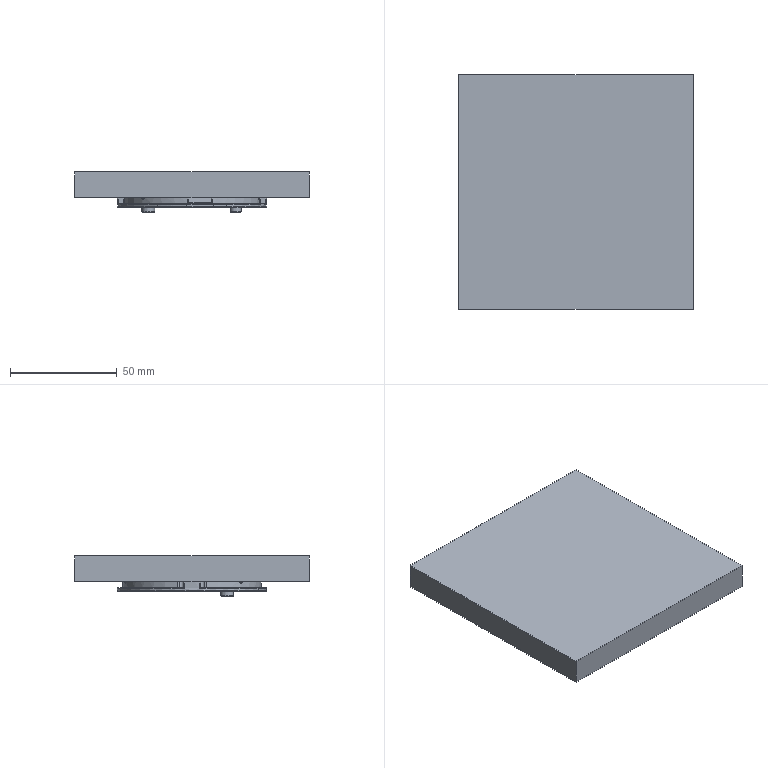NC program | NX | posted with a generic post | part box 110 x 110 x 18.8 mm
Lines 1 to 1072 of 3099:
N10 G17 G21 G94 G90
(FLOOR_WALL_COPY_1 , TOOL : D10)
N12 T04 M6
N14 G54
N16 G17 G0 G90 X-63. Y54.997 S6500 M3
N18 G43 Z30. H4
N20 Z3.
N22 G94 G1 Z0. F1250.
N24 X-60.
N26 X60.
N28 Y47.426
N30 X-60.
N32 Y39.855
N34 X60.
N36 Y32.283
N38 X-60.
N40 Y24.712
N42 X60.
N44 Y17.141
N46 X-60.
N48 Y9.57
N50 X60.
N52 Y1.999
N54 X-60.
N56 Y-5.573
N58 X60.
N60 Y-13.144
N62 X-60.
N64 Y-20.715
N66 X60.
N68 Y-28.286
N70 X-60.
N72 Y-35.858
N74 X60.
N76 Y-43.429
N78 X-60.
N80 Y-51.
N82 X60.
N84 X63.
N86 Z3.
N88 G0 Z30.
(FLOOR_WALL_COPY_1_COPY , TOOL : D10)
N90 X-20.7 Y1.195 S9500
N92 Z2.5
N94 G1 Y22.11 Z1.404 F1000.
N96 X-20.385 Y23.534 Z1.327
N98 X-19.742 Y24.842 Z1.251
N100 X-18.809 Y25.962 Z1.174
N102 X-18.329 Y26.332 Z1.143
N104 X-18.112 Y26.5 Z1.128
N106 X-26.5 Z0.689
N108 Y0. Z-0.7
N110 Y-26.5 F2500.
N112 X-19.233
N114 G2 X-20.7 Y-22.532 R6.1
N116 G1 Y21.505
N118 G2 X-18.329 Y26.332 R6.1
N120 G1 X-18.112 Y26.5
N122 X-26.5
N124 Y0.
N126 X-31.
N128 Y-31.
N130 X3.393
N132 X9.837 Y-33.606
N134 X3.393 Y-31.
N136 X-15.163 Y-24.03
N138 G2 X-16.2 Y-22.532 R1.6
N140 G1 Y21.505
N142 G2 X-15.578 Y22.771 R1.6
N144 G1 X-4.926 Y31.
N146 X-3.948 Y29.734
N148 X1.111 Y33.642
N150 X3.111 Y33.456
N152 G2 X12.353 Y-31.247 R33.6
N154 G1 X10.525 Y-31.97
N156 X-14.6 Y-22.532
N158 Y21.505
N160 X-3.948 Y29.734
N162 X-4.926 Y31.
N164 X-31.
N166 Y0.
N168 X-39.
N170 Y-39.
N172 X16.675
N174 Y-31.
N176 X31.
N178 Y-16.675
N180 X33.692 Y-11.317
N182 X31. Y-16.675
N184 G2 X16.675 Y-31. R35.2
N186 G1 Y-39.
N188 X39.
N190 Y16.675
N192 X31.
N194 Y31.
N196 X16.675
N198 X11.317 Y33.692
N200 X16.675 Y31.
N202 G2 X31. Y16.675 R35.2
N204 G1 X33.692 Y11.317
N206 X31. Y16.675
N208 X39.
N210 Y39.
N212 X-39.
N214 Y0.
N216 X-47.
N218 Y-47.
N220 X47.
N222 Y47.
N224 X-47.
N226 Y0.
N228 X-55.
N230 Y-47.988
N232 Y-55.
N234 X55.
N236 Y55.
N238 X-55.
N240 Y0.
N242 Z0.8
N244 G0 X-20.7 Y1.199
N246 G1 Y21.505 Z-0.264 F1000.
N248 Y22.11 Z-0.296
N250 X-20.389 Y23.521 Z-0.372
N252 X-19.879 Y24.62 Z-0.435
N254 X-19.391 Y25.329 Z-0.48
N256 X-18.809 Y25.962 Z-0.525
N258 X-18.112 Y26.5 Z-0.572
N260 X-26.5 Z-1.011
N262 Y0. Z-2.4
N264 Y-26.5 F2500.
N266 X-19.233
N268 G2 X-20.7 Y-22.532 R6.1
N270 G1 Y21.505
N272 G2 X-18.329 Y26.332 R6.1
N274 G1 X-18.112 Y26.5
N276 X-26.5
N278 Y0.
N280 X-31.
N282 Y-31.
N284 X3.393
N286 X9.837 Y-33.606
N288 X3.393 Y-31.
N290 X-15.163 Y-24.03
N292 G2 X-16.2 Y-22.532 R1.6
N294 G1 Y21.505
N296 G2 X-15.578 Y22.771 R1.6
N298 G1 X-4.926 Y31.
N300 X-3.948 Y29.734
N302 X1.111 Y33.642
N304 X3.111 Y33.456
N306 G2 X12.353 Y-31.247 R33.6
N308 G1 X10.525 Y-31.97
N310 X-14.6 Y-22.532
N312 Y21.505
N314 X-3.948 Y29.734
N316 X-4.926 Y31.
N318 X-31.
N320 Y0.
N322 X-39.
N324 Y-39.
N326 X16.675
N328 Y-31.
N330 X31.
N332 Y-16.675
N334 X33.692 Y-11.317
N336 X31. Y-16.675
N338 G2 X16.675 Y-31. R35.2
N340 G1 Y-39.
N342 X39.
N344 Y16.675
N346 X31.
N348 Y31.
N350 X16.675
N352 X11.317 Y33.692
N354 X16.675 Y31.
N356 G2 X31. Y16.675 R35.2
N358 G1 X33.692 Y11.317
N360 X31. Y16.675
N362 X39.
N364 Y39.
N366 X-39.
N368 Y0.
N370 X-47.
N372 Y-47.
N374 X47.
N376 Y47.
N378 X-47.
N380 Y0.
N382 X-55.
N384 Y-55.
N386 X55.
N388 Y55.
N390 X-55.
N392 Y0.
N394 Z-0.9
N396 G0 Z30.
(CAVITY_MILL_COPY , TOOL : D10)
N398 X-20.6 Y-3.644
N400 Z-1.
N402 G1 Y5.416 Z-1.475 F1000.
N404 X-20.888 Y4.322 Z-1.534
N406 X-21.281 Y1.45 Z-1.686
N408 Y-1.45 Z-1.838
N410 X-20.888 Y-4.322 Z-1.99
N412 X-20.6 Y-5.416 Z-2.049
N414 Y5.416 Z-2.617
N416 X-20.888 Y4.322 Z-2.676
N418 X-21.281 Y1.45 Z-2.828
N420 Y-1.45 Z-2.98
N422 X-20.888 Y-4.322 Z-3.132
N424 X-20.6 Y-5.416 Z-3.191
N426 Y0. Z-3.475
N428 Y5.416 F3000.
N430 X-19.652 Y10.432
N432 X-20.6 Y5.416
N434 G3 X-20.6 Y-5.416 R21.3
N436 G1 X-19.652 Y-10.432
N438 X-20.6 Y-5.416
N440 Y0.
N442 X-14.6
N444 Y19.
N446 G2 X-12.618 Y23.036 R5.1
N448 G1 X-9.136 Y25.726
N450 G3 X-2.128 Y-27.217 R27.3
N452 G1 X-11.293 Y-23.774
N454 G2 X-14.6 Y-19. R5.1
N456 G1 Y0.
N458 G3 X-15.1 Y0.866 R1.
N460 G1 Z-1.975
N462 G0 Z30.
N464 X-20.6 Y-3.644
N466 Z-1.975
N468 G1 Y5.416 Z-2.45 F1000.
N470 X-20.888 Y4.322 Z-2.509
N472 X-21.281 Y1.45 Z-2.661
N474 Y-1.45 Z-2.813
N476 X-20.888 Y-4.322 Z-2.965
N478 X-20.6 Y-5.416 Z-3.024
N480 Y5.416 Z-3.592
N482 X-20.888 Y4.322 Z-3.651
N484 X-21.281 Y1.45 Z-3.803
N486 Y-1.45 Z-3.955
N488 X-20.888 Y-4.322 Z-4.107
N490 X-20.6 Y-5.416 Z-4.166
N492 Y0. Z-4.45
N494 Y5.416 F3000.
N496 X-19.652 Y10.432
N498 X-20.6 Y5.416
N500 G3 X-20.6 Y-5.416 R21.3
N502 G1 X-19.652 Y-10.432
N504 X-20.6 Y-5.416
N506 Y0.
N508 X-14.6
N510 Y19.
N512 G2 X-12.618 Y23.036 R5.1
N514 G1 X-9.136 Y25.726
N516 G3 X-2.128 Y-27.217 R27.3
N518 G1 X-11.293 Y-23.774
N520 G2 X-14.6 Y-19. R5.1
N522 G1 Y0.
N524 G3 X-15.1 Y0.866 R1.
N526 G1 Z-2.95
N528 G0 X-20.6 Y-3.644
N530 G1 Y5.416 Z-3.425 F1000.
N532 X-20.888 Y4.322 Z-3.484
N534 X-21.281 Y1.45 Z-3.636
N536 Y-1.45 Z-3.788
N538 X-20.888 Y-4.322 Z-3.94
N540 X-20.6 Y-5.416 Z-3.999
N542 Y5.416 Z-4.567
N544 X-20.888 Y4.322 Z-4.626
N546 X-21.281 Y1.45 Z-4.778
N548 Y-1.45 Z-4.93
N550 X-20.888 Y-4.322 Z-5.082
N552 X-20.6 Y-5.416 Z-5.141
N554 Y0. Z-5.425
N556 Y5.416 F3000.
N558 X-19.652 Y10.432
N560 X-20.6 Y5.416
N562 G3 X-20.6 Y-5.416 R21.3
N564 G1 X-19.652 Y-10.432
N566 X-20.6 Y-5.416
N568 Y0.
N570 X-14.6
N572 Y19.
N574 G2 X-12.618 Y23.036 R5.1
N576 G1 X-9.136 Y25.726
N578 G3 X-2.128 Y-27.217 R27.3
N580 G1 X-11.293 Y-23.774
N582 G2 X-14.6 Y-19. R5.1
N584 G1 Y0.
N586 G3 X-15.1 Y0.866 R1.
N588 G1 Z-3.925
N590 G0 X-20.6 Y-3.644
N592 G1 Y5.416 Z-4.4 F1000.
N594 X-20.888 Y4.322 Z-4.459
N596 X-21.281 Y1.45 Z-4.611
N598 Y-1.45 Z-4.763
N600 X-20.888 Y-4.322 Z-4.915
N602 X-20.6 Y-5.416 Z-4.974
N604 Y5.416 Z-5.542
N606 X-20.888 Y4.322 Z-5.601
N608 X-21.281 Y1.45 Z-5.753
N610 Y-1.45 Z-5.905
N612 X-20.888 Y-4.322 Z-6.057
N614 X-20.6 Y-5.416 Z-6.116
N616 Y0. Z-6.4
N618 Y5.416 F3000.
N620 X-19.652 Y10.432
N622 X-20.6 Y5.416
N624 G3 X-20.6 Y-5.416 R21.3
N626 G1 X-19.652 Y-10.432
N628 X-20.6 Y-5.416
N630 Y0.
N632 X-14.6
N634 Y19.
N636 G2 X-12.618 Y23.036 R5.1
N638 G1 X-9.136 Y25.726
N640 G3 X-2.128 Y-27.217 R27.3
N642 G1 X-11.293 Y-23.774
N644 G2 X-14.6 Y-19. R5.1
N646 G1 Y0.
N648 G3 X-15.1 Y0.866 R1.
N650 G1 Z-4.9
N652 G0 X-16.803 Y-13.9
N654 G1 X-14.6 Z-5.015 F1000.
N656 Y13.9 Z-6.472
N658 X-18.4 Z-6.672
N660 Y0. Z-7.4
N662 Y-13.9 F3000.
N664 X-14.6
N666 Y13.9
N668 X-18.4
N670 Y0.
N672 G3 X-17.9 Y-0.866 R1.
N674 G1 Z-5.9
N676 G0 X-16.803 Y-13.9
N678 G1 X-14.6 Z-6.015 F1000.
N680 Y13.9 Z-7.472
N682 X-18.4 Z-7.672
N684 Y0. Z-8.4
N686 Y-13.9 F3000.
N688 X-14.6
N690 Y13.9
N692 X-18.4
N694 Y0.
N696 G3 X-17.9 Y-0.866 R1.
N698 G1 Z-6.9
N700 G0 X-16.803 Y-13.9
N702 G1 X-14.6 Z-7.015 F1000.
N704 Y13.9 Z-8.472
N706 X-18.4 Z-8.672
N708 Y0. Z-9.4
N710 Y-13.9 F3000.
N712 X-14.6
N714 Y13.9
N716 X-18.4
N718 Y0.
N720 G3 X-17.9 Y-0.866 R1.
N722 G1 Z-7.9
N724 G0 X-16.803 Y-13.9
N726 G1 X-14.6 Z-8.015 F1000.
N728 Y13.9 Z-9.472
N730 X-18.4 Z-9.672
N732 Y0. Z-10.4
N734 Y-13.9 F3000.
N736 X-14.6
N738 Y13.9
N740 X-18.4
N742 Y0.
N744 G3 X-17.9 Y-0.866 R1.
N746 G1 Z-8.9
N748 G0 X-16.803 Y-13.9
N750 G1 X-14.6 Z-9.015 F1000.
N752 Y13.9 Z-10.472
N754 X-18.4 Z-10.672
N756 Y0. Z-11.4
N758 Y-13.9 F3000.
N760 X-14.6
N762 Y13.9
N764 X-18.4
N766 Y0.
N768 G3 X-17.9 Y-0.866 R1.
N770 G1 Z-9.9
N772 G0 Z30.
N774 M5
(CAVITY_MILL_COPY_1_COPY_1 , TOOL : D6)
N776 T16 M6
N778 G54
N780 G17 G0 G90 X-2.983 Y-28.042 S9500 M3
N782 G43 Z30. H16
N784 Z-2.
N786 G94 G1 Z-3. F1000.
N788 X-2.607 Y-28.795
N790 G3 X-1.773 Y-29.347 R1.
N792 X7.243 Y-28.494 R29.4 F1600.
N794 G1 X-0.959 Y-25.413
N796 G3 X-1.946 Y-25.576 R1.
N798 G1 X-2.57 Y-26.089
N800 Z-2.
N802 G0 Z30.
N804 X-2.983 Y-28.042
N806 Z-2.5
N808 G1 Z-3.5 F1000.
N810 X-2.607 Y-28.795
N812 G3 X-1.773 Y-29.347 R1.
N814 X7.243 Y-28.494 R29.4 F1600.
N816 G1 X-0.959 Y-25.413
N818 G3 X-1.946 Y-25.576 R1.
N820 G1 X-2.57 Y-26.089
N822 Z-2.5
N824 G0 X-2.983 Y-28.042 Z-3.
N826 G1 Z-4. F1000.
N828 X-2.607 Y-28.795
N830 G3 X-1.773 Y-29.347 R1.
N832 X7.243 Y-28.494 R29.4 F1600.
N834 G1 X-0.959 Y-25.413
N836 G3 X-1.946 Y-25.576 R1.
N838 G1 X-2.57 Y-26.089
N840 Z-3.
N842 G0 X-2.983 Y-28.042 Z-3.5
N844 G1 Z-4.5 F1000.
N846 X-2.607 Y-28.795
N848 G3 X-1.773 Y-29.347 R1.
N850 X7.243 Y-28.494 R29.4 F1600.
N852 G1 X-0.959 Y-25.413
N854 G3 X-1.946 Y-25.576 R1.
N856 G1 X-2.57 Y-26.089
N858 Z-3.5
N860 G0 X-2.983 Y-28.042 Z-4.
N862 G1 Z-5. F1000.
N864 X-2.607 Y-28.795
N866 G3 X-1.773 Y-29.347 R1.
N868 X7.243 Y-28.494 R29.4 F1600.
N870 G1 X-0.959 Y-25.413
N872 G3 X-1.946 Y-25.576 R1.
N874 G1 X-2.57 Y-26.089
N876 Z-4.
N878 G0 X-2.983 Y-28.042 Z-4.5
N880 G1 Z-5.5 F1000.
N882 X-2.607 Y-28.795
N884 G3 X-1.773 Y-29.347 R1.
N886 X7.243 Y-28.494 R29.4 F1600.
N888 G1 X-0.959 Y-25.413
N890 G3 X-1.946 Y-25.576 R1.
N892 G1 X-2.57 Y-26.089
N894 Z-4.5
N896 G0 X-2.983 Y-28.042 Z-5.
N898 G1 Z-6. F1000.
N900 X-2.607 Y-28.795
N902 G3 X-1.773 Y-29.347 R1.
N904 X7.243 Y-28.494 R29.4 F1600.
N906 G1 X-0.959 Y-25.413
N908 G3 X-1.946 Y-25.576 R1.
N910 G1 X-2.57 Y-26.089
N912 Z-5.
N914 G0 X-2.983 Y-28.042 Z-5.5
N916 G1 Z-6.5 F1000.
N918 X-2.607 Y-28.795
N920 G3 X-1.773 Y-29.347 R1.
N922 X7.243 Y-28.494 R29.4 F1600.
N924 G1 X-0.959 Y-25.413
N926 G3 X-1.946 Y-25.576 R1.
N928 G1 X-2.57 Y-26.089
N930 Z-5.5
N932 G0 Z30.
N934 X-15.987 Y-14.8
N936 Z-6.
N938 G1 Z-7. F1000.
N940 X-15.582 Y-15.5
N942 G3 X-14.716 Y-16. R1.
N944 G1 X-12.5 F1600.
N946 Y-13.784
N948 G3 X-13. Y-12.918 R1.
N950 G1 X-13.7 Y-12.513
N952 Z-6.
N954 G0 X-15.987 Y-14.8 Z-6.5
N956 G1 Z-7.5 F1000.
N958 X-15.582 Y-15.5
N960 G3 X-14.716 Y-16. R1.
N962 G1 X-12.5 F1600.
N964 Y-13.784
N966 G3 X-13. Y-12.918 R1.
N968 G1 X-13.7 Y-12.513
N970 Z-6.5
N972 G0 X-15.987 Y-14.8 Z-7.
N974 G1 Z-8. F1000.
N976 X-15.582 Y-15.5
N978 G3 X-14.716 Y-16. R1.
N980 G1 X-12.5 F1600.
N982 Y-13.784
N984 G3 X-13. Y-12.918 R1.
N986 G1 X-13.7 Y-12.513
N988 Z-7.
N990 G0 X-15.987 Y-14.8 Z-7.5
N992 G1 Z-8.5 F1000.
N994 X-15.582 Y-15.5
N996 G3 X-14.716 Y-16. R1.
N998 G1 X-12.5 F1600.
N1000 Y-13.784
N1002 G3 X-13. Y-12.918 R1.
N1004 G1 X-13.7 Y-12.513
N1006 Z-7.5
N1008 G0 X-15.987 Y-14.8 Z-8.
N1010 G1 Z-9. F1000.
N1012 X-15.582 Y-15.5
N1014 G3 X-14.716 Y-16. R1.
N1016 G1 X-12.5 F1600.
N1018 Y-13.784
N1020 G3 X-13. Y-12.918 R1.
N1022 G1 X-13.7 Y-12.513
N1024 Z-8.
N1026 G0 X-15.987 Y-14.8 Z-8.5
N1028 G1 Z-9.5 F1000.
N1030 X-15.582 Y-15.5
N1032 G3 X-14.716 Y-16. R1.
N1034 G1 X-12.5 F1600.
N1036 Y-13.784
N1038 G3 X-13. Y-12.918 R1.
N1040 G1 X-13.7 Y-12.513
N1042 Z-8.5
N1044 G0 X-15.987 Y-14.8 Z-9.
N1046 G1 Z-10. F1000.
N1048 X-15.582 Y-15.5
N1050 G3 X-14.716 Y-16. R1.
N1052 G1 X-12.5 F1600.
N1054 Y-13.784
N1056 G3 X-13. Y-12.918 R1.
N1058 G1 X-13.7 Y-12.513
N1060 Z-9.
N1062 G0 X-15.987 Y-14.8 Z-9.5
N1064 G1 Z-10.5 F1000.
N1066 X-15.582 Y-15.5
N1068 G3 X-14.716 Y-16. R1.
N1070 G1 X-12.5 F1600.
N1072 Y-13.784
N1074 G3 X-13. Y-12.918 R1.
N1076 G1 X-13.7 Y-12.513
N1078 Z-9.5
N1080 G0 X-15.987 Y-14.8 Z-10.
N1082 G1 Z-11. F1000.
N1084 X-15.582 Y-15.5
N1086 G3 X-14.716 Y-16. R1.
N1088 G1 X-12.5 F1600.
N1090 Y-13.784
N1092 G3 X-13. Y-12.918 R1.
N1094 G1 X-13.7 Y-12.513
N1096 Z-10.
N1098 G0 X-15.987 Y-14.8 Z-10.5
N1100 G1 Z-11.5 F1000.
N1102 X-15.582 Y-15.5
N1104 G3 X-14.716 Y-16. R1.
N1106 G1 X-12.5 F1600.
N1108 Y-13.784
N1110 G3 X-13. Y-12.918 R1.
N1112 G1 X-13.7 Y-12.513
N1114 Z-10.5
N1116 G0 Z30.
N1118 X-19.3
N1120 Z-6.
N1122 G1 Z-7. F1000.
N1124 X-20. Y-12.917
N1126 G3 X-20.5 Y-13.783 R1.
N1128 G1 Y-16. F1600.
N1130 X-18.283
N1132 G3 X-17.417 Y-15.5 R1.
N1134 G1 X-17.013 Y-14.8
N1136 Z-6.
N1138 G0 X-19.3 Y-12.513 Z-6.5
N1140 G1 Z-7.5 F1000.
N1142 X-20. Y-12.917
N1144 G3 X-20.5 Y-13.783 R1.
N1146 G1 Y-16. F1600.
N1148 X-18.283
N1150 G3 X-17.417 Y-15.5 R1.
N1152 G1 X-17.013 Y-14.8
N1154 Z-6.5
N1156 G0 X-19.3 Y-12.513 Z-7.
N1158 G1 Z-8. F1000.
N1160 X-20. Y-12.917
N1162 G3 X-20.5 Y-13.783 R1.
N1164 G1 Y-16. F1600.
N1166 X-18.283
N1168 G3 X-17.417 Y-15.5 R1.
N1170 G1 X-17.013 Y-14.8
N1172 Z-7.
N1174 G0 X-19.3 Y-12.513 Z-7.5
N1176 G1 Z-8.5 F1000.
N1178 X-20. Y-12.917
N1180 G3 X-20.5 Y-13.783 R1.
N1182 G1 Y-16. F1600.
N1184 X-18.283
N1186 G3 X-17.417 Y-15.5 R1.
N1188 G1 X-17.013 Y-14.8
N1190 Z-7.5
N1192 G0 X-19.3 Y-12.513 Z-8.
N1194 G1 Z-9. F1000.
N1196 X-20. Y-12.917
N1198 G3 X-20.5 Y-13.783 R1.
N1200 G1 Y-16. F1600.
N1202 X-18.283
N1204 G3 X-17.417 Y-15.5 R1.
N1206 G1 X-17.013 Y-14.8
N1208 Z-8.
N1210 G0 X-19.3 Y-12.513 Z-8.5
N1212 G1 Z-9.5 F1000.
N1214 X-20. Y-12.917
N1216 G3 X-20.5 Y-13.783 R1.
N1218 G1 X-20.499 Y-16. F1600.
N1220 X-18.283
N1222 G3 X-17.417 Y-15.5 R1.
N1224 G1 X-17.013 Y-14.8
N1226 Z-8.5
N1228 G0 X-19.3 Y-12.513 Z-9.
N1230 G1 Z-10. F1000.
N1232 X-20. Y-12.917
N1234 G3 X-20.5 Y-13.783 R1.
N1236 G1 X-20.499 Y-16. F1600.
N1238 X-18.283
N1240 G3 X-17.417 Y-15.5 R1.
N1242 G1 X-17.013 Y-14.8
N1244 Z-9.
N1246 G0 X-19.3 Y-12.513 Z-9.5
N1248 G1 Z-10.5 F1000.
N1250 X-20. Y-12.917
N1252 G3 X-20.5 Y-13.783 R1.
N1254 G1 X-20.499 Y-16. F1600.
N1256 X-18.283
N1258 G3 X-17.417 Y-15.5 R1.
N1260 G1 X-17.013 Y-14.8
N1262 Z-9.5
N1264 G0 X-19.3 Y-12.513 Z-10.
N1266 G1 Z-11. F1000.
N1268 X-20. Y-12.917
N1270 G3 X-20.5 Y-13.783 R1.
N1272 G1 X-20.499 Y-16. F1600.
N1274 X-18.283
N1276 G3 X-17.417 Y-15.5 R1.
N1278 G1 X-17.013 Y-14.8
N1280 Z-10.
N1282 G0 X-19.3 Y-12.513 Z-10.5
N1284 G1 Z-11.5 F1000.
N1286 X-20. Y-12.917
N1288 G3 X-20.5 Y-13.783 R1.
N1290 G1 X-20.499 Y-16. F1600.
N1292 X-18.283
N1294 G3 X-17.417 Y-15.5 R1.
N1296 G1 X-17.013 Y-14.8
N1298 Z-10.5
N1300 G0 Z30.
N1302 Y14.8
N1304 Z-6.
N1306 G1 Z-7. F1000.
N1308 X-17.418 Y15.5
N1310 G3 X-18.284 Y16. R1.
N1312 G1 X-20.5 F1600.
N1314 Y13.784
N1316 G3 X-20. Y12.918 R1.
N1318 G1 X-19.3 Y12.513
N1320 Z-6.
N1322 G0 X-17.013 Y14.8 Z-6.5
N1324 G1 Z-7.5 F1000.
N1326 X-17.418 Y15.5
N1328 G3 X-18.284 Y16. R1.
N1330 G1 X-20.5 F1600.
N1332 Y13.784
N1334 G3 X-20. Y12.918 R1.
N1336 G1 X-19.3 Y12.513
N1338 Z-6.5
N1340 G0 X-17.013 Y14.8 Z-7.
N1342 G1 Z-8. F1000.
N1344 X-17.418 Y15.5
N1346 G3 X-18.284 Y16. R1.
N1348 G1 X-20.5 F1600.
N1350 Y13.784
N1352 G3 X-20. Y12.918 R1.
N1354 G1 X-19.3 Y12.513
N1356 Z-7.
N1358 G0 X-17.013 Y14.8 Z-7.5
N1360 G1 Z-8.5 F1000.
N1362 X-17.418 Y15.5
N1364 G3 X-18.284 Y16. R1.
N1366 G1 X-20.5 F1600.
N1368 Y13.784
N1370 G3 X-20. Y12.918 R1.
N1372 G1 X-19.3 Y12.513
N1374 Z-7.5
N1376 G0 X-17.013 Y14.8 Z-8.
N1378 G1 Z-9. F1000.
N1380 X-17.418 Y15.5
N1382 G3 X-18.284 Y16. R1.
N1384 G1 X-20.5 F1600.
N1386 Y13.784
N1388 G3 X-20. Y12.918 R1.
N1390 G1 X-19.3 Y12.513
N1392 Z-8.
N1394 G0 X-17.013 Y14.8 Z-8.5
N1396 G1 Z-9.5 F1000.
N1398 X-17.418 Y15.5
N1400 G3 X-18.284 Y16. R1.
N1402 G1 X-20.5 F1600.
N1404 Y13.784
N1406 G3 X-20. Y12.918 R1.
N1408 G1 X-19.3 Y12.513
N1410 Z-8.5
N1412 G0 X-17.013 Y14.8 Z-9.
N1414 G1 Z-10. F1000.
N1416 X-17.418 Y15.5
N1418 G3 X-18.284 Y16. R1.
N1420 G1 X-20.5 F1600.
N1422 Y13.784
N1424 G3 X-20. Y12.918 R1.
N1426 G1 X-19.3 Y12.513
N1428 Z-9.
N1430 G0 X-17.013 Y14.8 Z-9.5
N1432 G1 Z-10.5 F1000.
N1434 X-17.418 Y15.5
N1436 G3 X-18.284 Y16. R1.
N1438 G1 X-20.5 F1600.
N1440 Y13.784
N1442 G3 X-20. Y12.918 R1.
N1444 G1 X-19.3 Y12.513
N1446 Z-9.5
N1448 G0 X-17.013 Y14.8 Z-10.
N1450 G1 Z-11. F1000.
N1452 X-17.418 Y15.5
N1454 G3 X-18.284 Y16. R1.
N1456 G1 X-20.5 F1600.
N1458 Y13.784
N1460 G3 X-20. Y12.918 R1.
N1462 G1 X-19.3 Y12.513
N1464 Z-10.
N1466 G0 X-17.013 Y14.8 Z-10.5
N1468 G1 Z-11.5 F1000.
N1470 X-17.418 Y15.5
N1472 G3 X-18.284 Y16. R1.
N1474 G1 X-20.5 F1600.
N1476 Y13.784
N1478 G3 X-20. Y12.918 R1.
N1480 G1 X-19.3 Y12.513
N1482 Z-10.5
N1484 G0 Z30.
N1486 X-13.7
N1488 Z-6.
N1490 G1 Z-7. F1000.
N1492 X-13. Y12.918
N1494 G3 X-12.5 Y13.784 R1.
N1496 G1 Y16. F1600.
N1498 X-14.716
N1500 G3 X-15.582 Y15.5 R1.
N1502 G1 X-15.987 Y14.8
N1504 Z-6.
N1506 G0 X-13.7 Y12.513 Z-6.5
N1508 G1 Z-7.5 F1000.
N1510 X-13. Y12.918
N1512 G3 X-12.5 Y13.784 R1.
N1514 G1 Y16. F1600.
N1516 X-14.716
N1518 G3 X-15.582 Y15.5 R1.
N1520 G1 X-15.987 Y14.8
N1522 Z-6.5
N1524 G0 X-13.7 Y12.513 Z-7.
N1526 G1 Z-8. F1000.
N1528 X-13. Y12.918
N1530 G3 X-12.5 Y13.784 R1.
N1532 G1 Y16. F1600.
N1534 X-14.716
N1536 G3 X-15.582 Y15.5 R1.
N1538 G1 X-15.987 Y14.8
N1540 Z-7.
N1542 G0 X-13.7 Y12.513 Z-7.5
N1544 G1 Z-8.5 F1000.
N1546 X-13. Y12.918
N1548 G3 X-12.5 Y13.784 R1.
N1550 G1 Y16. F1600.
N1552 X-14.716
N1554 G3 X-15.582 Y15.5 R1.
N1556 G1 X-15.987 Y14.8
N1558 Z-7.5
N1560 G0 X-13.7 Y12.513 Z-8.
N1562 G1 Z-9. F1000.
N1564 X-13. Y12.918
N1566 G3 X-12.5 Y13.784 R1.
N1568 G1 Y16. F1600.
N1570 X-14.716
N1572 G3 X-15.582 Y15.5 R1.
N1574 G1 X-15.987 Y14.8
N1576 Z-8.
N1578 G0 X-13.7 Y12.513 Z-8.5
N1580 G1 Z-9.5 F1000.
N1582 X-13. Y12.918
N1584 G3 X-12.5 Y13.784 R1.
N1586 G1 Y16. F1600.
N1588 X-14.716
N1590 G3 X-15.582 Y15.5 R1.
N1592 G1 X-15.987 Y14.8
N1594 Z-8.5
N1596 G0 X-13.7 Y12.513 Z-9.
N1598 G1 Z-10. F1000.
N1600 X-13. Y12.918
N1602 G3 X-12.5 Y13.784 R1.
N1604 G1 Y16. F1600.
N1606 X-14.716
N1608 G3 X-15.582 Y15.5 R1.
N1610 G1 X-15.987 Y14.8
N1612 Z-9.
N1614 G0 X-13.7 Y12.513 Z-9.5
N1616 G1 Z-10.5 F1000.
N1618 X-13. Y12.918
N1620 G3 X-12.5 Y13.784 R1.
N1622 G1 Y16. F1600.
N1624 X-14.716
N1626 G3 X-15.582 Y15.5 R1.
N1628 G1 X-15.987 Y14.8
N1630 Z-9.5
N1632 G0 X-13.7 Y12.513 Z-10.
N1634 G1 Z-11. F1000.
N1636 X-13. Y12.918
N1638 G3 X-12.5 Y13.784 R1.
N1640 G1 Y16. F1600.
N1642 X-14.716
N1644 G3 X-15.582 Y15.5 R1.
N1646 G1 X-15.987 Y14.8
N1648 Z-10.
N1650 G0 X-13.7 Y12.513 Z-10.5
N1652 G1 Z-11.5 F1000.
N1654 X-13. Y12.918
N1656 G3 X-12.5 Y13.784 R1.
N1658 G1 Y16. F1600.
N1660 X-14.716
N1662 G3 X-15.582 Y15.5 R1.
N1664 G1 X-15.987 Y14.8
N1666 Z-10.5
N1668 G0 Z30.
N1670 X-9.283 Y24.475
N1672 Z-2.
N1674 G1 Z-3. F1000.
N1676 X-8.535 Y24.168
N1678 G3 X-7.544 Y24.302 R1.
N1680 G1 X-0.965 Y29.384 F1600.
N1682 G3 X-9.419 Y27.85 R29.4
N1684 X-10.079 Y27.099 R1.
N1686 G1 X-10.244 Y26.274
N1688 Z-2.
N1690 G0 Z30.
N1692 X-9.283 Y24.475
N1694 Z-2.5
N1696 G1 Z-3.5 F1000.
N1698 X-8.535 Y24.168
N1700 G3 X-7.544 Y24.302 R1.
N1702 G1 X-0.965 Y29.384 F1600.
N1704 G3 X-9.419 Y27.85 R29.4
N1706 X-10.079 Y27.099 R1.
N1708 G1 X-10.244 Y26.274
N1710 Z-2.5
N1712 G0 X-9.283 Y24.475 Z-3.
N1714 G1 Z-4. F1000.
N1716 X-8.535 Y24.168
N1718 G3 X-7.544 Y24.302 R1.
N1720 G1 X-0.965 Y29.384 F1600.
N1722 G3 X-9.419 Y27.85 R29.4
N1724 X-10.079 Y27.099 R1.
N1726 G1 X-10.244 Y26.274
N1728 Z-3.
N1730 G0 X-9.283 Y24.475 Z-3.5
N1732 G1 Z-4.5 F1000.
N1734 X-8.535 Y24.168
N1736 G3 X-7.544 Y24.302 R1.
N1738 G1 X-0.965 Y29.384 F1600.
N1740 G3 X-9.419 Y27.85 R29.4
N1742 X-10.079 Y27.099 R1.
N1744 G1 X-10.244 Y26.274
N1746 Z-3.5
N1748 G0 X-9.283 Y24.475 Z-4.
N1750 G1 Z-5. F1000.
N1752 X-8.535 Y24.168
N1754 G3 X-7.544 Y24.302 R1.
N1756 G1 X-0.965 Y29.384 F1600.
N1758 G3 X-9.419 Y27.85 R29.4
N1760 X-10.079 Y27.099 R1.
N1762 G1 X-10.244 Y26.274
N1764 Z-4.
N1766 G0 X-9.283 Y24.475 Z-4.5
N1768 G1 Z-5.5 F1000.
N1770 X-8.535 Y24.168
N1772 G3 X-7.544 Y24.302 R1.
N1774 G1 X-0.965 Y29.384 F1600.
N1776 G3 X-9.419 Y27.85 R29.4
N1778 X-10.079 Y27.099 R1.
N1780 G1 X-10.244 Y26.274
N1782 Z-4.5
N1784 G0 X-9.283 Y24.475 Z-5.
N1786 G1 Z-6. F1000.
N1788 X-8.535 Y24.168
N1790 G3 X-7.544 Y24.302 R1.
N1792 G1 X-0.965 Y29.384 F1600.
N1794 G3 X-9.419 Y27.85 R29.4
N1796 X-10.079 Y27.099 R1.
N1798 G1 X-10.244 Y26.274
N1800 Z-5.
N1802 G0 X-9.283 Y24.475 Z-5.5
N1804 G1 Z-6.5 F1000.
N1806 X-8.535 Y24.168
N1808 G3 X-7.544 Y24.302 R1.
N1810 G1 X-0.965 Y29.384 F1600.
N1812 G3 X-9.419 Y27.85 R29.4
N1814 X-10.079 Y27.099 R1.
N1816 G1 X-10.244 Y26.274
N1818 Z-5.5
N1820 G0 Z30.
(FLOOR_WALL_1_COPY_COPY , TOOL : D6)
N1822 X-59.5 Y-1.212
N1824 Z-1.
N1826 G1 Z-2.5 F1000.
N1828 X-58.3 Y-0.52
N1830 G3 X-58. Y0. R0.6
N1832 G1 Y58.
N1834 X58.
N1836 Y-58.
N1838 X-58.
N1840 Y0.
N1842 X-55.
N1844 Y55.
N1846 X55.
N1848 Y-55.
N1850 X-55.
N1852 Y0.
N1854 X-52.
N1856 Y52.
N1858 X52.
N1860 Y-52.
N1862 X-52.
N1864 Y0.
N1866 X-49.
N1868 Y49.
N1870 X49.
N1872 Y-49.
N1874 X-49.
N1876 Y0.
N1878 X-46.
N1880 Y46.
N1882 X46.
N1884 Y-46.
N1886 X-46.
N1888 Y0.
N1890 X-43.
N1892 Y43.
N1894 X43.
N1896 Y-43.
N1898 X-43.
N1900 Y0.
N1902 X-40.
N1904 Y40.
N1906 X40.
N1908 Y-40.
N1910 X-40.
N1912 Y0.
N1914 X-37.
N1916 Y37.
N1918 X37.
N1920 Y-37.
N1922 X-37.
N1924 Y0.
N1926 X-34.
N1928 Y34.
N1930 X34.
N1932 Y9.76
N1934 X31.
N1936 G3 X9.76 Y31. R32.5
N1938 G1 X31.
N1940 Y21.823
N1942 X28.
N1944 G3 X21.823 Y28. R35.5
N1946 G1 X28.
N1948 Y21.823
N1950 X31.
N1952 Y9.76
N1954 X34.
N1956 Y-34.
N1958 X-34.
N1960 Y0.
N1962 X-31.
N1964 Y31.
N1966 X-0.509
N1968 X-13.15 Y21.235
N1970 G3 X-13.5 Y20.522 R0.9
N1972 G1 Y-21.147
N1974 G3 X-12.916 Y-21.99 R0.9
N1976 G1 X10.19 Y-30.669
N1978 G3 X10.837 Y-30.663 R0.9
N1980 G1 X11.948 Y-30.224
N1982 G3 X31. Y-9.76 R32.5
N1984 G1 X30.428 Y-9.579
N1986 G2 X11.728 Y-29.666 R31.9
N1988 G1 X10.617 Y-30.105
N1990 G2 X10.401 Y-30.107 R0.3
N1992 G1 X-12.705 Y-21.428
N1994 G2 X-12.9 Y-21.147 R0.3
N1996 G1 Y20.522
N1998 G2 X-12.783 Y20.76 R0.3
N2000 G1 X1.527 Y31.815
N2002 G2 X1.738 Y31.876 R0.3
N2004 G1 X2.954 Y31.763
N2006 G2 X30.428 Y-9.579 R31.9
N2008 G1 X31. Y-9.76
N2010 Y-31.
N2012 X21.823
N2014 Y-28.
N2016 G3 X28. Y-21.823 R35.5
N2018 G1 Y-28.
N2020 X21.823
N2022 Y-31.
N2024 X-31.
N2026 Y0.
N2028 X-28.
N2030 Y28.
N2032 X-9.3
N2034 X-14.984 Y23.609
N2036 G3 X-16.5 Y20.522 R3.9
N2038 G1 Y-21.147
N2040 G3 X-13.971 Y-24.798 R3.9
N2042 G1 X-5.447 Y-28.
N2044 X-28.
N2046 Y0.
N2048 X-25.
N2050 Y25.
N2052 X-17.85
N2054 G3 X-19.5 Y20.522 R6.9
N2056 G1 Y-21.147
N2058 G3 X-18.324 Y-25. R6.9
N2060 G1 X-25.
N2062 Y0.
N2064 X-22.3
N2066 Y22.3
N2068 X-22.034
N2070 G3 X-22.2 Y20.522 R9.6
N2072 G1 Y-21.147
N2074 G3 X-22.131 Y-22.3 R9.6
N2076 G1 X-22.3
N2078 Y0.
N2080 G3 X-22.6 Y0.52 R0.6
N2082 G1 Z-1.
N2084 G0 Z30.
N2086 X-14.4 Y-1.698
N2088 Z-1.
N2090 G1 Z-2.5
N2092 X-12.9 Y-0.832
N2094 G3 X-12.6 Y-0.312 R0.6
N2096 G1 Y20.522
N2098 X1.71 Y31.577
N2100 X2.926 Y31.464
N2102 G2 X11.617 Y-29.387 R31.6
N2104 G1 X10.506 Y-29.826
N2106 X-12.6 Y-21.147
N2108 Y-0.312
N2110 G3 X-12.9 Y0.207 R0.6
N2112 G1 X-14.4 Y1.073
N2114 Z-1.
N2116 G0 Z30.
N2118 M5